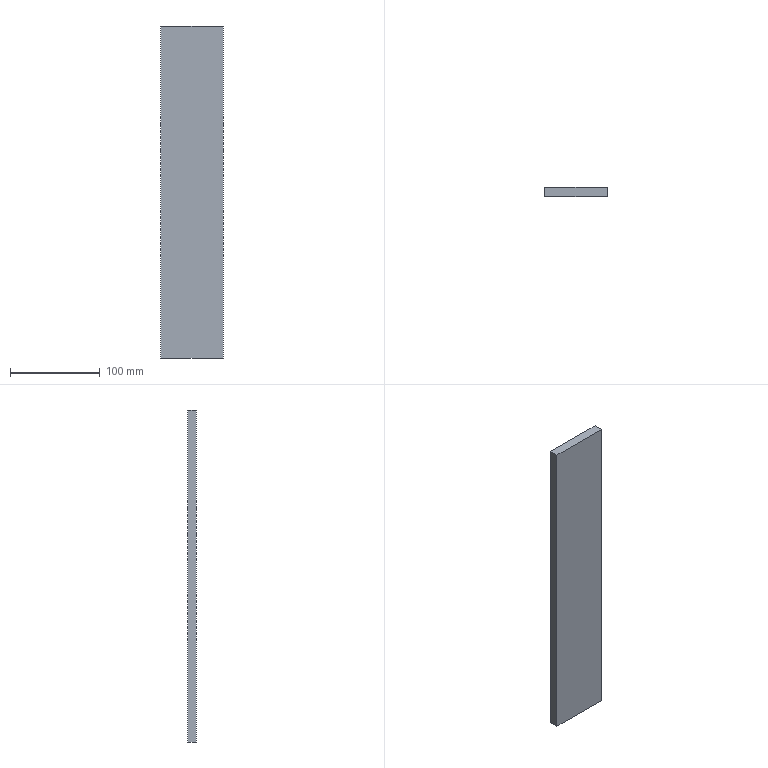Part | NX | features solid 2 | 1 solid | 6 faces | box 70 x 10 x 370 mm | volume 259000 mm3 | plane 6
STEP:
#1=CARTESIAN_POINT('',(-1060.,0.,-110.));
#2=VERTEX_POINT('',#1);
#3=CARTESIAN_POINT('',(-1060.,10.,-110.));
#4=VERTEX_POINT('',#3);
#5=CARTESIAN_POINT('',(-1060.,0.,-110.));
#6=DIRECTION('',(0.,1.,0.));
#7=VECTOR('',#6,1000.);
#8=LINE('',#5,#7);
#9=EDGE_CURVE('',#2,#4,#8,.T.);
#10=ORIENTED_EDGE('',*,*,#9,.T.);
#11=CARTESIAN_POINT('',(-1060.,10.,-480.));
#12=VERTEX_POINT('',#11);
#13=CARTESIAN_POINT('',(-1060.,10.,-15.));
#14=DIRECTION('',(0.,0.,1.));
#15=VECTOR('',#14,1000.);
#16=LINE('',#13,#15);
#17=EDGE_CURVE('',#12,#4,#16,.T.);
#18=ORIENTED_EDGE('',*,*,#17,.F.);
#19=CARTESIAN_POINT('',(-1060.,0.,-480.));
#20=VERTEX_POINT('',#19);
#21=CARTESIAN_POINT('',(-1060.,0.,-480.));
#22=DIRECTION('',(0.,-1.,0.));
#23=VECTOR('',#22,1000.);
#24=LINE('',#21,#23);
#25=EDGE_CURVE('',#12,#20,#24,.T.);
#26=ORIENTED_EDGE('',*,*,#25,.T.);
#27=CARTESIAN_POINT('',(-1060.,0.,-15.));
#28=DIRECTION('',(0.,0.,1.));
#29=VECTOR('',#28,1000.);
#30=LINE('',#27,#29);
#31=EDGE_CURVE('',#20,#2,#30,.T.);
#32=ORIENTED_EDGE('',*,*,#31,.T.);
#33=EDGE_LOOP('',(#10,#18,#26,#32));
#34=FACE_BOUND('',#33,.T.);
#35=CARTESIAN_POINT('',(-1060.,0.,-15.));
#36=DIRECTION('',(1.,0.,0.));
#37=DIRECTION('',(0.,-1.,0.));
#38=AXIS2_PLACEMENT_3D('',#35,#36,#37);
#39=PLANE('',#38);
#40=ADVANCED_FACE('',(#34),#39,.F.);
#41=CARTESIAN_POINT('',(-990.,0.,-110.));
#42=VERTEX_POINT('',#41);
#43=CARTESIAN_POINT('',(-990.,10.,-110.));
#44=VERTEX_POINT('',#43);
#45=CARTESIAN_POINT('',(-990.,10.,-110.));
#46=DIRECTION('',(0.,1.,0.));
#47=VECTOR('',#46,1000.);
#48=LINE('',#45,#47);
#49=EDGE_CURVE('',#42,#44,#48,.T.);
#50=ORIENTED_EDGE('',*,*,#49,.T.);
#51=CARTESIAN_POINT('',(-990.,10.,-110.));
#52=DIRECTION('',(1.,0.,0.));
#53=VECTOR('',#52,1000.);
#54=LINE('',#51,#53);
#55=EDGE_CURVE('',#4,#44,#54,.T.);
#56=ORIENTED_EDGE('',*,*,#55,.F.);
#57=ORIENTED_EDGE('',*,*,#9,.F.);
#58=CARTESIAN_POINT('',(-990.,0.,-110.));
#59=DIRECTION('',(1.,0.,0.));
#60=VECTOR('',#59,1000.);
#61=LINE('',#58,#60);
#62=EDGE_CURVE('',#2,#42,#61,.T.);
#63=ORIENTED_EDGE('',*,*,#62,.T.);
#64=EDGE_LOOP('',(#50,#56,#57,#63));
#65=FACE_BOUND('',#64,.T.);
#66=CARTESIAN_POINT('',(-990.,10.,-110.));
#67=DIRECTION('',(0.,0.,-1.));
#68=DIRECTION('',(0.,-1.,0.));
#69=AXIS2_PLACEMENT_3D('',#66,#67,#68);
#70=PLANE('',#69);
#71=ADVANCED_FACE('',(#65),#70,.F.);
#72=ORIENTED_EDGE('',*,*,#17,.T.);
#73=ORIENTED_EDGE('',*,*,#55,.T.);
#74=CARTESIAN_POINT('',(-990.,10.,-480.));
#75=VERTEX_POINT('',#74);
#76=CARTESIAN_POINT('',(-990.,10.,-480.));
#77=DIRECTION('',(0.,0.,-1.));
#78=VECTOR('',#77,1000.);
#79=LINE('',#76,#78);
#80=EDGE_CURVE('',#44,#75,#79,.T.);
#81=ORIENTED_EDGE('',*,*,#80,.T.);
#82=CARTESIAN_POINT('',(-990.,10.,-480.));
#83=DIRECTION('',(-1.,0.,0.));
#84=VECTOR('',#83,1000.);
#85=LINE('',#82,#84);
#86=EDGE_CURVE('',#75,#12,#85,.T.);
#87=ORIENTED_EDGE('',*,*,#86,.T.);
#88=EDGE_LOOP('',(#72,#73,#81,#87));
#89=FACE_BOUND('',#88,.T.);
#90=CARTESIAN_POINT('',(-990.,10.,-480.));
#91=DIRECTION('',(0.,1.,0.));
#92=DIRECTION('',(1.,0.,0.));
#93=AXIS2_PLACEMENT_3D('',#90,#91,#92);
#94=PLANE('',#93);
#95=ADVANCED_FACE('',(#89),#94,.T.);
#96=ORIENTED_EDGE('',*,*,#25,.F.);
#97=ORIENTED_EDGE('',*,*,#86,.F.);
#98=CARTESIAN_POINT('',(-990.,0.,-480.));
#99=VERTEX_POINT('',#98);
#100=CARTESIAN_POINT('',(-990.,0.,-480.));
#101=DIRECTION('',(0.,-1.,0.));
#102=VECTOR('',#101,1000.);
#103=LINE('',#100,#102);
#104=EDGE_CURVE('',#75,#99,#103,.T.);
#105=ORIENTED_EDGE('',*,*,#104,.T.);
#106=CARTESIAN_POINT('',(-990.,0.,-480.));
#107=DIRECTION('',(-1.,0.,0.));
#108=VECTOR('',#107,1000.);
#109=LINE('',#106,#108);
#110=EDGE_CURVE('',#99,#20,#109,.T.);
#111=ORIENTED_EDGE('',*,*,#110,.T.);
#112=EDGE_LOOP('',(#96,#97,#105,#111));
#113=FACE_BOUND('',#112,.T.);
#114=CARTESIAN_POINT('',(-990.,0.,-480.));
#115=DIRECTION('',(0.,0.,1.));
#116=DIRECTION('',(1.,0.,0.));
#117=AXIS2_PLACEMENT_3D('',#114,#115,#116);
#118=PLANE('',#117);
#119=ADVANCED_FACE('',(#113),#118,.F.);
#120=ORIENTED_EDGE('',*,*,#62,.F.);
#121=ORIENTED_EDGE('',*,*,#31,.F.);
#122=ORIENTED_EDGE('',*,*,#110,.F.);
#123=CARTESIAN_POINT('',(-990.,0.,-480.));
#124=DIRECTION('',(0.,0.,1.));
#125=VECTOR('',#124,1000.);
#126=LINE('',#123,#125);
#127=EDGE_CURVE('',#99,#42,#126,.T.);
#128=ORIENTED_EDGE('',*,*,#127,.T.);
#129=EDGE_LOOP('',(#120,#121,#122,#128));
#130=FACE_BOUND('',#129,.T.);
#131=CARTESIAN_POINT('',(-990.,0.,-480.));
#132=DIRECTION('',(0.,1.,0.));
#133=DIRECTION('',(1.,0.,0.));
#134=AXIS2_PLACEMENT_3D('',#131,#132,#133);
#135=PLANE('',#134);
#136=ADVANCED_FACE('',(#130),#135,.F.);
#137=ORIENTED_EDGE('',*,*,#104,.F.);
#138=ORIENTED_EDGE('',*,*,#80,.F.);
#139=ORIENTED_EDGE('',*,*,#49,.F.);
#140=ORIENTED_EDGE('',*,*,#127,.F.);
#141=EDGE_LOOP('',(#137,#138,#139,#140));
#142=FACE_BOUND('',#141,.T.);
#143=CARTESIAN_POINT('',(-990.,0.,-480.));
#144=DIRECTION('',(-1.,0.,0.));
#145=DIRECTION('',(0.,0.,1.));
#146=AXIS2_PLACEMENT_3D('',#143,#144,#145);
#147=PLANE('',#146);
#148=ADVANCED_FACE('',(#142),#147,.F.);
#149=CLOSED_SHELL('',(#40,#71,#95,#119,#136,#148));
#150=MANIFOLD_SOLID_BREP('',#149);
#151=(LENGTH_UNIT()NAMED_UNIT(*)SI_UNIT(.MILLI.,.METRE.));
#152=UNCERTAINTY_MEASURE_WITH_UNIT(LENGTH_MEASURE(0.00001),#151,'','');
#153=(NAMED_UNIT(*)PLANE_ANGLE_UNIT()SI_UNIT($,.RADIAN.));
#154=(NAMED_UNIT(*)SI_UNIT($,.STERADIAN.)SOLID_ANGLE_UNIT());
#155=(GEOMETRIC_REPRESENTATION_CONTEXT(3)GLOBAL_UNCERTAINTY_ASSIGNED_CONTEXT((#152))GLOBAL_UNIT_ASSIGNED_CONTEXT((#151,#153,#154))REPRESENTATION_CONTEXT('',''));
#156=ADVANCED_BREP_SHAPE_REPRESENTATION('',(#150),#155);